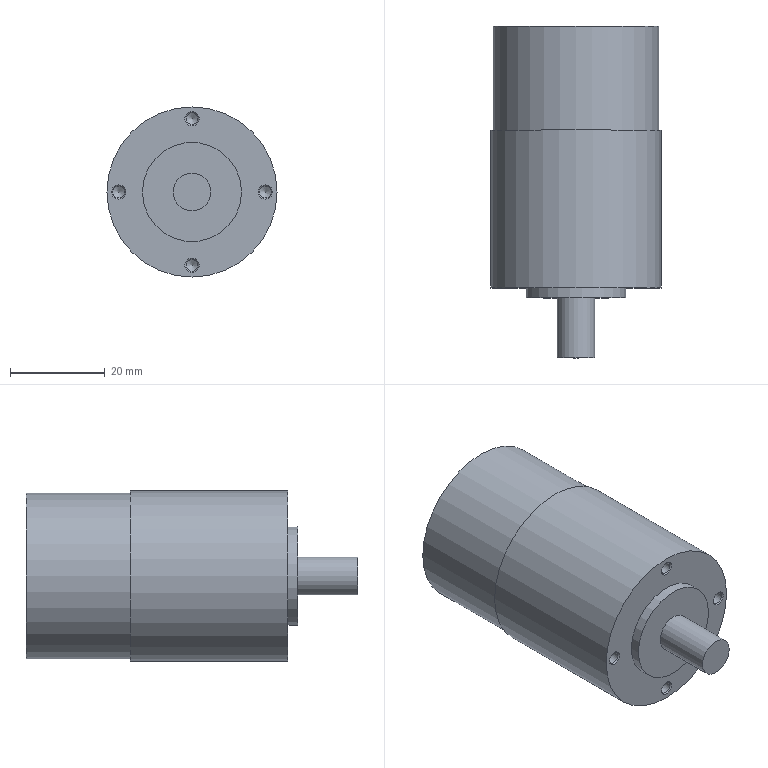Part | NX | features DATUM_CSYS 6, SKETCH 5, EXTRUDE 4, SIMPLE HOLE 4, SYMBOLIC_THREAD 4, HOLE PACKAGE 1 | 1 solid | 21 faces | box 36 x 70.2 x 36 mm | volume 56405 mm3 | cylinder 8 | cone 8 | plane 5 | commonest cylinder face diameters 2.5 x4 8 x1 21 x1 35 x1 36 x1
STEP:
#1=CARTESIAN_POINT('',(17.5,-22.,0.));
#2=VERTEX_POINT('',#1);
#3=CARTESIAN_POINT('',(0.,-22.,0.));
#4=DIRECTION('',(0.,-1.,0.));
#5=DIRECTION('',(1.,0.,0.));
#6=AXIS2_PLACEMENT_3D('',#3,#4,#5);
#7=CIRCLE('',#6,17.5);
#8=EDGE_CURVE('',#2,#2,#7,.T.);
#9=ORIENTED_EDGE('',*,*,#8,.F.);
#10=EDGE_LOOP('',(#9));
#11=FACE_BOUND('',#10,.T.);
#12=CARTESIAN_POINT('',(17.5,0.,0.));
#13=VERTEX_POINT('',#12);
#14=CARTESIAN_POINT('',(0.,0.,0.));
#15=DIRECTION('',(0.,-1.,0.));
#16=DIRECTION('',(1.,0.,0.));
#17=AXIS2_PLACEMENT_3D('',#14,#15,#16);
#18=CIRCLE('',#17,17.5);
#19=EDGE_CURVE('',#13,#13,#18,.T.);
#20=ORIENTED_EDGE('',*,*,#19,.T.);
#21=EDGE_LOOP('',(#20));
#22=FACE_BOUND('',#21,.T.);
#23=CARTESIAN_POINT('',(0.,-22.,0.));
#24=DIRECTION('',(0.,1.,0.));
#25=DIRECTION('',(0.,0.,1.));
#26=AXIS2_PLACEMENT_3D('',#23,#24,#25);
#27=CYLINDRICAL_SURFACE('',#26,17.5);
#28=ADVANCED_FACE('',(#11,#22),#27,.T.);
#29=ORIENTED_EDGE('',*,*,#19,.F.);
#30=EDGE_LOOP('',(#29));
#31=FACE_BOUND('',#30,.T.);
#32=CARTESIAN_POINT('',(0.,0.,0.));
#33=DIRECTION('',(0.,-1.,0.));
#34=DIRECTION('',(0.,0.,-1.));
#35=AXIS2_PLACEMENT_3D('',#32,#33,#34);
#36=PLANE('',#35);
#37=ADVANCED_FACE('',(#31),#36,.F.);
#38=CARTESIAN_POINT('',(18.,-55.4,0.));
#39=VERTEX_POINT('',#38);
#40=CARTESIAN_POINT('',(0.,-55.4,0.));
#41=DIRECTION('',(0.,-1.,0.));
#42=DIRECTION('',(1.,0.,0.));
#43=AXIS2_PLACEMENT_3D('',#40,#41,#42);
#44=CIRCLE('',#43,18.);
#45=EDGE_CURVE('',#39,#39,#44,.T.);
#46=ORIENTED_EDGE('',*,*,#45,.F.);
#47=EDGE_LOOP('',(#46));
#48=FACE_BOUND('',#47,.T.);
#49=CARTESIAN_POINT('',(18.,-22.,0.));
#50=VERTEX_POINT('',#49);
#51=CARTESIAN_POINT('',(0.,-22.,0.));
#52=DIRECTION('',(0.,-1.,0.));
#53=DIRECTION('',(1.,0.,0.));
#54=AXIS2_PLACEMENT_3D('',#51,#52,#53);
#55=CIRCLE('',#54,18.);
#56=EDGE_CURVE('',#50,#50,#55,.T.);
#57=ORIENTED_EDGE('',*,*,#56,.T.);
#58=EDGE_LOOP('',(#57));
#59=FACE_BOUND('',#58,.T.);
#60=CARTESIAN_POINT('',(0.,-55.4,0.));
#61=DIRECTION('',(0.,1.,0.));
#62=DIRECTION('',(0.,0.,1.));
#63=AXIS2_PLACEMENT_3D('',#60,#61,#62);
#64=CYLINDRICAL_SURFACE('',#63,18.);
#65=ADVANCED_FACE('',(#48,#59),#64,.T.);
#66=CARTESIAN_POINT('',(15.5,-55.4,-1.5));
#67=VERTEX_POINT('',#66);
#68=CARTESIAN_POINT('',(15.5,-55.4,0.));
#69=DIRECTION('',(0.,-1.,0.));
#70=DIRECTION('',(0.,0.,-1.));
#71=AXIS2_PLACEMENT_3D('',#68,#69,#70);
#72=CIRCLE('',#71,1.5);
#73=EDGE_CURVE('',#67,#67,#72,.F.);
#74=ORIENTED_EDGE('',*,*,#73,.T.);
#75=EDGE_LOOP('',(#74));
#76=FACE_BOUND('',#75,.T.);
#77=CARTESIAN_POINT('',(0.,-55.4,14.));
#78=VERTEX_POINT('',#77);
#79=CARTESIAN_POINT('',(0.,-55.4,15.5));
#80=DIRECTION('',(0.,-1.,0.));
#81=DIRECTION('',(0.,0.,-1.));
#82=AXIS2_PLACEMENT_3D('',#79,#80,#81);
#83=CIRCLE('',#82,1.5);
#84=EDGE_CURVE('',#78,#78,#83,.F.);
#85=ORIENTED_EDGE('',*,*,#84,.T.);
#86=EDGE_LOOP('',(#85));
#87=FACE_BOUND('',#86,.T.);
#88=CARTESIAN_POINT('',(0.,-55.4,-17.));
#89=VERTEX_POINT('',#88);
#90=CARTESIAN_POINT('',(0.,-55.4,-15.5));
#91=DIRECTION('',(0.,-1.,0.));
#92=DIRECTION('',(0.,0.,-1.));
#93=AXIS2_PLACEMENT_3D('',#90,#91,#92);
#94=CIRCLE('',#93,1.5);
#95=EDGE_CURVE('',#89,#89,#94,.F.);
#96=ORIENTED_EDGE('',*,*,#95,.T.);
#97=EDGE_LOOP('',(#96));
#98=FACE_BOUND('',#97,.T.);
#99=CARTESIAN_POINT('',(-15.5,-55.4,-1.5));
#100=VERTEX_POINT('',#99);
#101=CARTESIAN_POINT('',(-15.5,-55.4,0.));
#102=DIRECTION('',(0.,-1.,0.));
#103=DIRECTION('',(0.,0.,-1.));
#104=AXIS2_PLACEMENT_3D('',#101,#102,#103);
#105=CIRCLE('',#104,1.5);
#106=EDGE_CURVE('',#100,#100,#105,.F.);
#107=ORIENTED_EDGE('',*,*,#106,.T.);
#108=EDGE_LOOP('',(#107));
#109=FACE_BOUND('',#108,.T.);
#110=CARTESIAN_POINT('',(10.5,-55.4,0.));
#111=VERTEX_POINT('',#110);
#112=CARTESIAN_POINT('',(0.,-55.4,0.));
#113=DIRECTION('',(0.,-1.,0.));
#114=DIRECTION('',(1.,0.,0.));
#115=AXIS2_PLACEMENT_3D('',#112,#113,#114);
#116=CIRCLE('',#115,10.5);
#117=EDGE_CURVE('',#111,#111,#116,.T.);
#118=ORIENTED_EDGE('',*,*,#117,.F.);
#119=EDGE_LOOP('',(#118));
#120=FACE_BOUND('',#119,.T.);
#121=ORIENTED_EDGE('',*,*,#45,.T.);
#122=EDGE_LOOP('',(#121));
#123=FACE_BOUND('',#122,.T.);
#124=CARTESIAN_POINT('',(0.,-55.4,0.));
#125=DIRECTION('',(0.,-1.,0.));
#126=DIRECTION('',(0.,0.,-1.));
#127=AXIS2_PLACEMENT_3D('',#124,#125,#126);
#128=PLANE('',#127);
#129=ADVANCED_FACE('',(#76,#87,#98,#109,#120,#123),#128,.T.);
#130=ORIENTED_EDGE('',*,*,#8,.T.);
#131=EDGE_LOOP('',(#130));
#132=FACE_BOUND('',#131,.T.);
#133=ORIENTED_EDGE('',*,*,#56,.F.);
#134=EDGE_LOOP('',(#133));
#135=FACE_BOUND('',#134,.T.);
#136=CARTESIAN_POINT('',(0.,-22.,0.));
#137=DIRECTION('',(0.,-1.,0.));
#138=DIRECTION('',(0.,0.,-1.));
#139=AXIS2_PLACEMENT_3D('',#136,#137,#138);
#140=PLANE('',#139);
#141=ADVANCED_FACE('',(#132,#135),#140,.F.);
#142=CARTESIAN_POINT('',(10.5,-57.5,0.));
#143=VERTEX_POINT('',#142);
#144=CARTESIAN_POINT('',(0.,-57.5,0.));
#145=DIRECTION('',(0.,-1.,0.));
#146=DIRECTION('',(1.,0.,0.));
#147=AXIS2_PLACEMENT_3D('',#144,#145,#146);
#148=CIRCLE('',#147,10.5);
#149=EDGE_CURVE('',#143,#143,#148,.T.);
#150=ORIENTED_EDGE('',*,*,#149,.F.);
#151=EDGE_LOOP('',(#150));
#152=FACE_BOUND('',#151,.T.);
#153=ORIENTED_EDGE('',*,*,#117,.T.);
#154=EDGE_LOOP('',(#153));
#155=FACE_BOUND('',#154,.T.);
#156=CARTESIAN_POINT('',(0.,-57.5,0.));
#157=DIRECTION('',(0.,1.,0.));
#158=DIRECTION('',(0.,0.,1.));
#159=AXIS2_PLACEMENT_3D('',#156,#157,#158);
#160=CYLINDRICAL_SURFACE('',#159,10.5);
#161=ADVANCED_FACE('',(#152,#155),#160,.T.);
#162=CARTESIAN_POINT('',(4.,-57.5,0.));
#163=VERTEX_POINT('',#162);
#164=CARTESIAN_POINT('',(0.,-57.5,0.));
#165=DIRECTION('',(0.,-1.,0.));
#166=DIRECTION('',(1.,0.,0.));
#167=AXIS2_PLACEMENT_3D('',#164,#165,#166);
#168=CIRCLE('',#167,4.);
#169=EDGE_CURVE('',#163,#163,#168,.T.);
#170=ORIENTED_EDGE('',*,*,#169,.F.);
#171=EDGE_LOOP('',(#170));
#172=FACE_BOUND('',#171,.T.);
#173=ORIENTED_EDGE('',*,*,#149,.T.);
#174=EDGE_LOOP('',(#173));
#175=FACE_BOUND('',#174,.T.);
#176=CARTESIAN_POINT('',(0.,-57.5,0.));
#177=DIRECTION('',(0.,-1.,0.));
#178=DIRECTION('',(0.,0.,-1.));
#179=AXIS2_PLACEMENT_3D('',#176,#177,#178);
#180=PLANE('',#179);
#181=ADVANCED_FACE('',(#172,#175),#180,.T.);
#182=CARTESIAN_POINT('',(4.,-70.2,0.));
#183=VERTEX_POINT('',#182);
#184=CARTESIAN_POINT('',(0.,-70.2,0.));
#185=DIRECTION('',(0.,-1.,0.));
#186=DIRECTION('',(1.,0.,0.));
#187=AXIS2_PLACEMENT_3D('',#184,#185,#186);
#188=CIRCLE('',#187,4.);
#189=EDGE_CURVE('',#183,#183,#188,.T.);
#190=ORIENTED_EDGE('',*,*,#189,.F.);
#191=EDGE_LOOP('',(#190));
#192=FACE_BOUND('',#191,.T.);
#193=ORIENTED_EDGE('',*,*,#169,.T.);
#194=EDGE_LOOP('',(#193));
#195=FACE_BOUND('',#194,.T.);
#196=CARTESIAN_POINT('',(0.,-70.2,0.));
#197=DIRECTION('',(0.,1.,0.));
#198=DIRECTION('',(0.,0.,1.));
#199=AXIS2_PLACEMENT_3D('',#196,#197,#198);
#200=CYLINDRICAL_SURFACE('',#199,4.);
#201=ADVANCED_FACE('',(#192,#195),#200,.T.);
#202=ORIENTED_EDGE('',*,*,#189,.T.);
#203=EDGE_LOOP('',(#202));
#204=FACE_BOUND('',#203,.T.);
#205=CARTESIAN_POINT('',(0.,-70.2,0.));
#206=DIRECTION('',(0.,-1.,0.));
#207=DIRECTION('',(0.,0.,-1.));
#208=AXIS2_PLACEMENT_3D('',#205,#206,#207);
#209=PLANE('',#208);
#210=ADVANCED_FACE('',(#204),#209,.T.);
#211=CARTESIAN_POINT('',(-15.5,-49.4,1.25));
#212=VERTEX_POINT('',#211);
#213=CARTESIAN_POINT('',(-15.5,-49.4,0.));
#214=DIRECTION('',(0.,1.,0.));
#215=DIRECTION('',(0.,0.,1.));
#216=AXIS2_PLACEMENT_3D('',#213,#214,#215);
#217=CIRCLE('',#216,1.25);
#218=EDGE_CURVE('',#212,#212,#217,.F.);
#219=ORIENTED_EDGE('',*,*,#218,.T.);
#220=EDGE_LOOP('',(#219));
#221=FACE_BOUND('',#220,.T.);
#222=CARTESIAN_POINT('',(-15.5,-48.649,0.));
#223=VERTEX_POINT('',#222);
#224=VERTEX_LOOP('',#223);
#225=FACE_BOUND('',#224,.T.);
#226=CARTESIAN_POINT('',(-15.5,-49.4,0.));
#227=DIRECTION('',(0.,-1.,0.));
#228=DIRECTION('',(0.,0.,-1.));
#229=AXIS2_PLACEMENT_3D('',#226,#227,#228);
#230=CONICAL_SURFACE('',#229,1.25,1.03);
#231=ADVANCED_FACE('',(#221,#225),#230,.F.);
#232=CARTESIAN_POINT('',(-15.5,-55.15,-1.25));
#233=VERTEX_POINT('',#232);
#234=CARTESIAN_POINT('',(-15.5,-55.15,0.));
#235=DIRECTION('',(0.,-1.,0.));
#236=DIRECTION('',(0.,0.,-1.));
#237=AXIS2_PLACEMENT_3D('',#234,#235,#236);
#238=CIRCLE('',#237,1.25);
#239=EDGE_CURVE('',#233,#233,#238,.T.);
#240=ORIENTED_EDGE('',*,*,#239,.T.);
#241=EDGE_LOOP('',(#240));
#242=FACE_BOUND('',#241,.T.);
#243=ORIENTED_EDGE('',*,*,#218,.F.);
#244=EDGE_LOOP('',(#243));
#245=FACE_BOUND('',#244,.T.);
#246=CARTESIAN_POINT('',(-15.5,-55.4,0.));
#247=DIRECTION('',(0.,1.,0.));
#248=DIRECTION('',(0.,0.,1.));
#249=AXIS2_PLACEMENT_3D('',#246,#247,#248);
#250=CYLINDRICAL_SURFACE('',#249,1.25);
#251=ADVANCED_FACE('',(#242,#245),#250,.F.);
#252=ORIENTED_EDGE('',*,*,#239,.F.);
#253=EDGE_LOOP('',(#252));
#254=FACE_BOUND('',#253,.T.);
#255=ORIENTED_EDGE('',*,*,#106,.F.);
#256=EDGE_LOOP('',(#255));
#257=FACE_BOUND('',#256,.T.);
#258=CARTESIAN_POINT('',(-15.5,-55.4,0.));
#259=DIRECTION('',(0.,-1.,0.));
#260=DIRECTION('',(0.,0.,-1.));
#261=AXIS2_PLACEMENT_3D('',#258,#259,#260);
#262=CONICAL_SURFACE('',#261,1.5,0.7854);
#263=ADVANCED_FACE('',(#254,#257),#262,.F.);
#264=CARTESIAN_POINT('',(0.,-49.4,-14.25));
#265=VERTEX_POINT('',#264);
#266=CARTESIAN_POINT('',(0.,-49.4,-15.5));
#267=DIRECTION('',(0.,1.,0.));
#268=DIRECTION('',(0.,0.,1.));
#269=AXIS2_PLACEMENT_3D('',#266,#267,#268);
#270=CIRCLE('',#269,1.25);
#271=EDGE_CURVE('',#265,#265,#270,.F.);
#272=ORIENTED_EDGE('',*,*,#271,.T.);
#273=EDGE_LOOP('',(#272));
#274=FACE_BOUND('',#273,.T.);
#275=CARTESIAN_POINT('',(0.,-48.649,-15.5));
#276=VERTEX_POINT('',#275);
#277=VERTEX_LOOP('',#276);
#278=FACE_BOUND('',#277,.T.);
#279=CARTESIAN_POINT('',(0.,-49.4,-15.5));
#280=DIRECTION('',(0.,-1.,0.));
#281=DIRECTION('',(0.,0.,-1.));
#282=AXIS2_PLACEMENT_3D('',#279,#280,#281);
#283=CONICAL_SURFACE('',#282,1.25,1.03);
#284=ADVANCED_FACE('',(#274,#278),#283,.F.);
#285=CARTESIAN_POINT('',(0.,-55.15,-16.75));
#286=VERTEX_POINT('',#285);
#287=CARTESIAN_POINT('',(0.,-55.15,-15.5));
#288=DIRECTION('',(0.,-1.,0.));
#289=DIRECTION('',(0.,0.,-1.));
#290=AXIS2_PLACEMENT_3D('',#287,#288,#289);
#291=CIRCLE('',#290,1.25);
#292=EDGE_CURVE('',#286,#286,#291,.T.);
#293=ORIENTED_EDGE('',*,*,#292,.T.);
#294=EDGE_LOOP('',(#293));
#295=FACE_BOUND('',#294,.T.);
#296=ORIENTED_EDGE('',*,*,#271,.F.);
#297=EDGE_LOOP('',(#296));
#298=FACE_BOUND('',#297,.T.);
#299=CARTESIAN_POINT('',(0.,-55.4,-15.5));
#300=DIRECTION('',(0.,1.,0.));
#301=DIRECTION('',(0.,0.,1.));
#302=AXIS2_PLACEMENT_3D('',#299,#300,#301);
#303=CYLINDRICAL_SURFACE('',#302,1.25);
#304=ADVANCED_FACE('',(#295,#298),#303,.F.);
#305=ORIENTED_EDGE('',*,*,#292,.F.);
#306=EDGE_LOOP('',(#305));
#307=FACE_BOUND('',#306,.T.);
#308=ORIENTED_EDGE('',*,*,#95,.F.);
#309=EDGE_LOOP('',(#308));
#310=FACE_BOUND('',#309,.T.);
#311=CARTESIAN_POINT('',(0.,-55.4,-15.5));
#312=DIRECTION('',(0.,-1.,0.));
#313=DIRECTION('',(0.,0.,-1.));
#314=AXIS2_PLACEMENT_3D('',#311,#312,#313);
#315=CONICAL_SURFACE('',#314,1.5,0.7854);
#316=ADVANCED_FACE('',(#307,#310),#315,.F.);
#317=CARTESIAN_POINT('',(0.,-49.4,16.75));
#318=VERTEX_POINT('',#317);
#319=CARTESIAN_POINT('',(0.,-49.4,15.5));
#320=DIRECTION('',(0.,1.,0.));
#321=DIRECTION('',(0.,0.,1.));
#322=AXIS2_PLACEMENT_3D('',#319,#320,#321);
#323=CIRCLE('',#322,1.25);
#324=EDGE_CURVE('',#318,#318,#323,.F.);
#325=ORIENTED_EDGE('',*,*,#324,.T.);
#326=EDGE_LOOP('',(#325));
#327=FACE_BOUND('',#326,.T.);
#328=CARTESIAN_POINT('',(0.,-48.649,15.5));
#329=VERTEX_POINT('',#328);
#330=VERTEX_LOOP('',#329);
#331=FACE_BOUND('',#330,.T.);
#332=CARTESIAN_POINT('',(0.,-49.4,15.5));
#333=DIRECTION('',(0.,-1.,0.));
#334=DIRECTION('',(0.,0.,-1.));
#335=AXIS2_PLACEMENT_3D('',#332,#333,#334);
#336=CONICAL_SURFACE('',#335,1.25,1.03);
#337=ADVANCED_FACE('',(#327,#331),#336,.F.);
#338=CARTESIAN_POINT('',(0.,-55.15,14.25));
#339=VERTEX_POINT('',#338);
#340=CARTESIAN_POINT('',(0.,-55.15,15.5));
#341=DIRECTION('',(0.,-1.,0.));
#342=DIRECTION('',(0.,0.,-1.));
#343=AXIS2_PLACEMENT_3D('',#340,#341,#342);
#344=CIRCLE('',#343,1.25);
#345=EDGE_CURVE('',#339,#339,#344,.T.);
#346=ORIENTED_EDGE('',*,*,#345,.T.);
#347=EDGE_LOOP('',(#346));
#348=FACE_BOUND('',#347,.T.);
#349=ORIENTED_EDGE('',*,*,#324,.F.);
#350=EDGE_LOOP('',(#349));
#351=FACE_BOUND('',#350,.T.);
#352=CARTESIAN_POINT('',(0.,-55.4,15.5));
#353=DIRECTION('',(0.,1.,0.));
#354=DIRECTION('',(0.,0.,1.));
#355=AXIS2_PLACEMENT_3D('',#352,#353,#354);
#356=CYLINDRICAL_SURFACE('',#355,1.25);
#357=ADVANCED_FACE('',(#348,#351),#356,.F.);
#358=ORIENTED_EDGE('',*,*,#345,.F.);
#359=EDGE_LOOP('',(#358));
#360=FACE_BOUND('',#359,.T.);
#361=ORIENTED_EDGE('',*,*,#84,.F.);
#362=EDGE_LOOP('',(#361));
#363=FACE_BOUND('',#362,.T.);
#364=CARTESIAN_POINT('',(0.,-55.4,15.5));
#365=DIRECTION('',(0.,-1.,0.));
#366=DIRECTION('',(0.,0.,-1.));
#367=AXIS2_PLACEMENT_3D('',#364,#365,#366);
#368=CONICAL_SURFACE('',#367,1.5,0.7854);
#369=ADVANCED_FACE('',(#360,#363),#368,.F.);
#370=CARTESIAN_POINT('',(15.5,-49.4,1.25));
#371=VERTEX_POINT('',#370);
#372=CARTESIAN_POINT('',(15.5,-49.4,0.));
#373=DIRECTION('',(0.,1.,0.));
#374=DIRECTION('',(0.,0.,1.));
#375=AXIS2_PLACEMENT_3D('',#372,#373,#374);
#376=CIRCLE('',#375,1.25);
#377=EDGE_CURVE('',#371,#371,#376,.F.);
#378=ORIENTED_EDGE('',*,*,#377,.T.);
#379=EDGE_LOOP('',(#378));
#380=FACE_BOUND('',#379,.T.);
#381=CARTESIAN_POINT('',(15.5,-48.649,0.));
#382=VERTEX_POINT('',#381);
#383=VERTEX_LOOP('',#382);
#384=FACE_BOUND('',#383,.T.);
#385=CARTESIAN_POINT('',(15.5,-49.4,0.));
#386=DIRECTION('',(0.,-1.,0.));
#387=DIRECTION('',(0.,0.,-1.));
#388=AXIS2_PLACEMENT_3D('',#385,#386,#387);
#389=CONICAL_SURFACE('',#388,1.25,1.03);
#390=ADVANCED_FACE('',(#380,#384),#389,.F.);
#391=CARTESIAN_POINT('',(15.5,-55.15,-1.25));
#392=VERTEX_POINT('',#391);
#393=CARTESIAN_POINT('',(15.5,-55.15,0.));
#394=DIRECTION('',(0.,-1.,0.));
#395=DIRECTION('',(0.,0.,-1.));
#396=AXIS2_PLACEMENT_3D('',#393,#394,#395);
#397=CIRCLE('',#396,1.25);
#398=EDGE_CURVE('',#392,#392,#397,.T.);
#399=ORIENTED_EDGE('',*,*,#398,.T.);
#400=EDGE_LOOP('',(#399));
#401=FACE_BOUND('',#400,.T.);
#402=ORIENTED_EDGE('',*,*,#377,.F.);
#403=EDGE_LOOP('',(#402));
#404=FACE_BOUND('',#403,.T.);
#405=CARTESIAN_POINT('',(15.5,-55.4,0.));
#406=DIRECTION('',(0.,1.,0.));
#407=DIRECTION('',(0.,0.,1.));
#408=AXIS2_PLACEMENT_3D('',#405,#406,#407);
#409=CYLINDRICAL_SURFACE('',#408,1.25);
#410=ADVANCED_FACE('',(#401,#404),#409,.F.);
#411=ORIENTED_EDGE('',*,*,#398,.F.);
#412=EDGE_LOOP('',(#411));
#413=FACE_BOUND('',#412,.T.);
#414=ORIENTED_EDGE('',*,*,#73,.F.);
#415=EDGE_LOOP('',(#414));
#416=FACE_BOUND('',#415,.T.);
#417=CARTESIAN_POINT('',(15.5,-55.4,0.));
#418=DIRECTION('',(0.,-1.,0.));
#419=DIRECTION('',(0.,0.,-1.));
#420=AXIS2_PLACEMENT_3D('',#417,#418,#419);
#421=CONICAL_SURFACE('',#420,1.5,0.7854);
#422=ADVANCED_FACE('',(#413,#416),#421,.F.);
#423=CLOSED_SHELL('',(#28,#37,#65,#129,#141,#161,#181,#201,#210,#231,#251,#263,#284,#304,#316,#337,#357,#369,#390,#410,#422));
#424=MANIFOLD_SOLID_BREP('',#423);
#425=(LENGTH_UNIT()NAMED_UNIT(*)SI_UNIT(.MILLI.,.METRE.));
#426=UNCERTAINTY_MEASURE_WITH_UNIT(LENGTH_MEASURE(0.00001),#425,'','');
#427=(NAMED_UNIT(*)PLANE_ANGLE_UNIT()SI_UNIT($,.RADIAN.));
#428=(NAMED_UNIT(*)SI_UNIT($,.STERADIAN.)SOLID_ANGLE_UNIT());
#429=(GEOMETRIC_REPRESENTATION_CONTEXT(3)GLOBAL_UNCERTAINTY_ASSIGNED_CONTEXT((#426))GLOBAL_UNIT_ASSIGNED_CONTEXT((#425,#427,#428))REPRESENTATION_CONTEXT('',''));
#430=ADVANCED_BREP_SHAPE_REPRESENTATION('',(#424),#429);